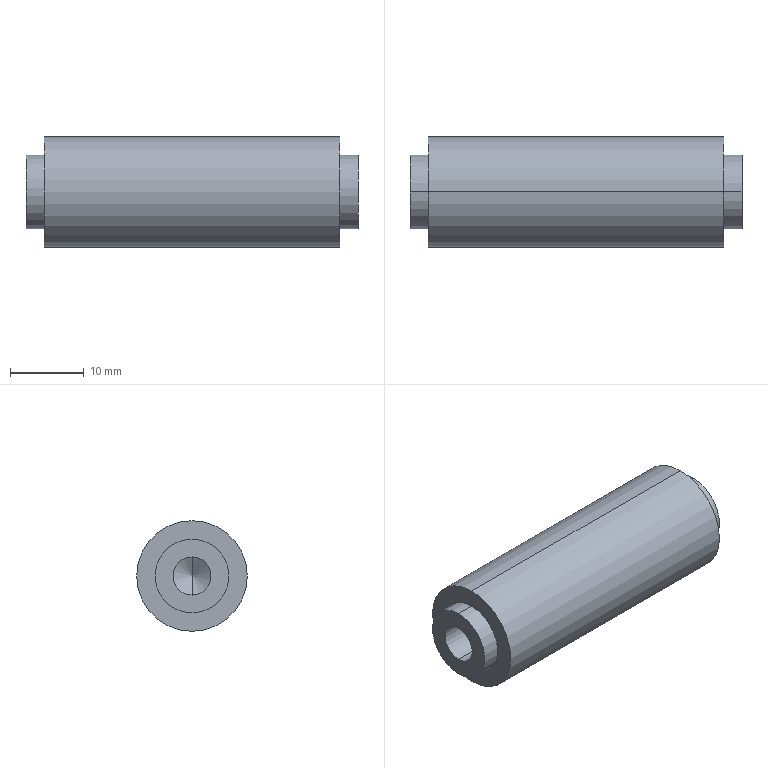Part | SolidWorks | features BaseBody 1 | 1 solid | 18 faces | box 45 x 15 x 15 mm | volume 6805 mm3 | cylinder 10 | cone 4 | plane 4 | commonest cylinder face diameters 5.188 x4 10 x4 15 x2
STEP:
#1=CARTESIAN_POINT('',(20.,0.,7.5));
#2=VERTEX_POINT('',#1);
#3=CARTESIAN_POINT('',(20.,0.,-7.5));
#4=VERTEX_POINT('',#3);
#5=CARTESIAN_POINT('',(20.,0.,0.));
#6=DIRECTION('',(-1.,0.,0.));
#7=DIRECTION('',(0.,0.,1.));
#8=AXIS2_PLACEMENT_3D('',#5,#6,#7);
#9=CIRCLE('',#8,7.5);
#10=EDGE_CURVE('',#2,#4,#9,.T.);
#11=ORIENTED_EDGE('',*,*,#10,.T.);
#12=CARTESIAN_POINT('',(-20.,0.,-7.5));
#13=VERTEX_POINT('',#12);
#14=CARTESIAN_POINT('',(20.,0.,-7.5));
#15=DIRECTION('',(-1.,0.,0.));
#16=VECTOR('',#15,1000.);
#17=LINE('',#14,#16);
#18=EDGE_CURVE('',#4,#13,#17,.T.);
#19=ORIENTED_EDGE('',*,*,#18,.T.);
#20=CARTESIAN_POINT('',(-20.,0.,7.5));
#21=VERTEX_POINT('',#20);
#22=CARTESIAN_POINT('',(-20.,0.,0.));
#23=DIRECTION('',(1.,0.,0.));
#24=DIRECTION('',(0.,0.,1.));
#25=AXIS2_PLACEMENT_3D('',#22,#23,#24);
#26=CIRCLE('',#25,7.5);
#27=EDGE_CURVE('',#13,#21,#26,.T.);
#28=ORIENTED_EDGE('',*,*,#27,.T.);
#29=CARTESIAN_POINT('',(20.,0.,7.5));
#30=DIRECTION('',(-1.,0.,0.));
#31=VECTOR('',#30,1000.);
#32=LINE('',#29,#31);
#33=EDGE_CURVE('',#2,#21,#32,.T.);
#34=ORIENTED_EDGE('',*,*,#33,.F.);
#35=EDGE_LOOP('',(#11,#19,#28,#34));
#36=FACE_OUTER_BOUND('',#35,.T.);
#37=CARTESIAN_POINT('',(20.,0.,0.));
#38=DIRECTION('',(-1.,0.,0.));
#39=DIRECTION('',(0.,0.,1.));
#40=AXIS2_PLACEMENT_3D('',#37,#38,#39);
#41=CYLINDRICAL_SURFACE('',#40,7.5);
#42=ADVANCED_FACE('',(#36),#41,.T.);
#43=CARTESIAN_POINT('',(-20.,0.,5.));
#44=VERTEX_POINT('',#43);
#45=CARTESIAN_POINT('',(-20.,0.,-5.));
#46=VERTEX_POINT('',#45);
#47=CARTESIAN_POINT('',(-20.,0.,0.));
#48=DIRECTION('',(-1.,0.,0.));
#49=DIRECTION('',(0.,0.,1.));
#50=AXIS2_PLACEMENT_3D('',#47,#48,#49);
#51=CIRCLE('',#50,5.);
#52=EDGE_CURVE('',#44,#46,#51,.T.);
#53=ORIENTED_EDGE('',*,*,#52,.T.);
#54=CARTESIAN_POINT('',(-22.5,0.,-5.));
#55=VERTEX_POINT('',#54);
#56=CARTESIAN_POINT('',(-20.,0.,-5.));
#57=DIRECTION('',(-1.,0.,0.));
#58=VECTOR('',#57,1000.);
#59=LINE('',#56,#58);
#60=EDGE_CURVE('',#46,#55,#59,.T.);
#61=ORIENTED_EDGE('',*,*,#60,.T.);
#62=CARTESIAN_POINT('',(-22.5,0.,5.));
#63=VERTEX_POINT('',#62);
#64=CARTESIAN_POINT('',(-22.5,0.,0.));
#65=DIRECTION('',(1.,0.,0.));
#66=DIRECTION('',(0.,0.,1.));
#67=AXIS2_PLACEMENT_3D('',#64,#65,#66);
#68=CIRCLE('',#67,5.);
#69=EDGE_CURVE('',#55,#63,#68,.T.);
#70=ORIENTED_EDGE('',*,*,#69,.T.);
#71=CARTESIAN_POINT('',(-20.,0.,5.));
#72=DIRECTION('',(-1.,0.,0.));
#73=VECTOR('',#72,1000.);
#74=LINE('',#71,#73);
#75=EDGE_CURVE('',#44,#63,#74,.T.);
#76=ORIENTED_EDGE('',*,*,#75,.F.);
#77=EDGE_LOOP('',(#53,#61,#70,#76));
#78=FACE_OUTER_BOUND('',#77,.T.);
#79=CARTESIAN_POINT('',(-20.,0.,0.));
#80=DIRECTION('',(-1.,0.,0.));
#81=DIRECTION('',(0.,0.,1.));
#82=AXIS2_PLACEMENT_3D('',#79,#80,#81);
#83=CYLINDRICAL_SURFACE('',#82,5.);
#84=ADVANCED_FACE('',(#78),#83,.T.);
#85=CARTESIAN_POINT('',(20.,0.,5.));
#86=VERTEX_POINT('',#85);
#87=CARTESIAN_POINT('',(20.,0.,-5.));
#88=VERTEX_POINT('',#87);
#89=CARTESIAN_POINT('',(20.,0.,0.));
#90=DIRECTION('',(-1.,0.,0.));
#91=DIRECTION('',(0.,0.,-1.));
#92=AXIS2_PLACEMENT_3D('',#89,#90,#91);
#93=CIRCLE('',#92,5.);
#94=EDGE_CURVE('',#86,#88,#93,.T.);
#95=ORIENTED_EDGE('',*,*,#94,.F.);
#96=CARTESIAN_POINT('',(22.5,0.,5.));
#97=VERTEX_POINT('',#96);
#98=CARTESIAN_POINT('',(20.,0.,5.));
#99=DIRECTION('',(1.,0.,0.));
#100=VECTOR('',#99,1000.);
#101=LINE('',#98,#100);
#102=EDGE_CURVE('',#86,#97,#101,.T.);
#103=ORIENTED_EDGE('',*,*,#102,.T.);
#104=CARTESIAN_POINT('',(22.5,0.,-5.));
#105=VERTEX_POINT('',#104);
#106=CARTESIAN_POINT('',(22.5,0.,0.));
#107=DIRECTION('',(-1.,0.,0.));
#108=DIRECTION('',(0.,0.,-1.));
#109=AXIS2_PLACEMENT_3D('',#106,#107,#108);
#110=CIRCLE('',#109,5.);
#111=EDGE_CURVE('',#97,#105,#110,.T.);
#112=ORIENTED_EDGE('',*,*,#111,.T.);
#113=CARTESIAN_POINT('',(20.,0.,-5.));
#114=DIRECTION('',(1.,0.,0.));
#115=VECTOR('',#114,1000.);
#116=LINE('',#113,#115);
#117=EDGE_CURVE('',#88,#105,#116,.T.);
#118=ORIENTED_EDGE('',*,*,#117,.F.);
#119=EDGE_LOOP('',(#95,#103,#112,#118));
#120=FACE_OUTER_BOUND('',#119,.T.);
#121=CARTESIAN_POINT('',(20.,0.,0.));
#122=DIRECTION('',(1.,0.,0.));
#123=DIRECTION('',(0.,0.,-1.));
#124=AXIS2_PLACEMENT_3D('',#121,#122,#123);
#125=CYLINDRICAL_SURFACE('',#124,5.);
#126=ADVANCED_FACE('',(#120),#125,.T.);
#127=CARTESIAN_POINT('',(-22.5,0.,2.594));
#128=VERTEX_POINT('',#127);
#129=CARTESIAN_POINT('',(-22.5,0.,-2.594));
#130=VERTEX_POINT('',#129);
#131=CARTESIAN_POINT('',(-22.5,0.,0.));
#132=DIRECTION('',(1.,0.,0.));
#133=DIRECTION('',(0.,0.,-1.));
#134=AXIS2_PLACEMENT_3D('',#131,#132,#133);
#135=CIRCLE('',#134,2.594);
#136=EDGE_CURVE('',#128,#130,#135,.T.);
#137=ORIENTED_EDGE('',*,*,#136,.F.);
#138=CARTESIAN_POINT('',(-7.5,0.,2.594));
#139=VERTEX_POINT('',#138);
#140=CARTESIAN_POINT('',(-22.5,0.,2.594));
#141=DIRECTION('',(1.,0.,0.));
#142=VECTOR('',#141,1000.);
#143=LINE('',#140,#142);
#144=EDGE_CURVE('',#128,#139,#143,.T.);
#145=ORIENTED_EDGE('',*,*,#144,.T.);
#146=CARTESIAN_POINT('',(-7.5,0.,-2.594));
#147=VERTEX_POINT('',#146);
#148=CARTESIAN_POINT('',(-7.5,0.,0.));
#149=DIRECTION('',(-1.,0.,0.));
#150=DIRECTION('',(0.,0.,-1.));
#151=AXIS2_PLACEMENT_3D('',#148,#149,#150);
#152=CIRCLE('',#151,2.594);
#153=EDGE_CURVE('',#147,#139,#152,.T.);
#154=ORIENTED_EDGE('',*,*,#153,.F.);
#155=CARTESIAN_POINT('',(-22.5,0.,-2.594));
#156=DIRECTION('',(1.,0.,0.));
#157=VECTOR('',#156,1000.);
#158=LINE('',#155,#157);
#159=EDGE_CURVE('',#130,#147,#158,.T.);
#160=ORIENTED_EDGE('',*,*,#159,.F.);
#161=EDGE_LOOP('',(#137,#145,#154,#160));
#162=FACE_OUTER_BOUND('',#161,.T.);
#163=CARTESIAN_POINT('',(-22.5,0.,0.));
#164=DIRECTION('',(1.,0.,0.));
#165=DIRECTION('',(0.,0.,-1.));
#166=AXIS2_PLACEMENT_3D('',#163,#164,#165);
#167=CYLINDRICAL_SURFACE('',#166,2.594);
#168=ADVANCED_FACE('',(#162),#167,.F.);
#169=CARTESIAN_POINT('',(22.5,0.,-2.594));
#170=VERTEX_POINT('',#169);
#171=CARTESIAN_POINT('',(22.5,0.,2.594));
#172=VERTEX_POINT('',#171);
#173=CARTESIAN_POINT('',(22.5,0.,0.));
#174=DIRECTION('',(-1.,0.,0.));
#175=DIRECTION('',(0.,0.,1.));
#176=AXIS2_PLACEMENT_3D('',#173,#174,#175);
#177=CIRCLE('',#176,2.594);
#178=EDGE_CURVE('',#170,#172,#177,.T.);
#179=ORIENTED_EDGE('',*,*,#178,.F.);
#180=CARTESIAN_POINT('',(7.5,0.,-2.594));
#181=VERTEX_POINT('',#180);
#182=CARTESIAN_POINT('',(22.5,0.,-2.594));
#183=DIRECTION('',(-1.,0.,0.));
#184=VECTOR('',#183,1000.);
#185=LINE('',#182,#184);
#186=EDGE_CURVE('',#170,#181,#185,.T.);
#187=ORIENTED_EDGE('',*,*,#186,.T.);
#188=CARTESIAN_POINT('',(7.5,0.,2.594));
#189=VERTEX_POINT('',#188);
#190=CARTESIAN_POINT('',(7.5,0.,0.));
#191=DIRECTION('',(1.,0.,0.));
#192=DIRECTION('',(0.,0.,1.));
#193=AXIS2_PLACEMENT_3D('',#190,#191,#192);
#194=CIRCLE('',#193,2.594);
#195=EDGE_CURVE('',#189,#181,#194,.T.);
#196=ORIENTED_EDGE('',*,*,#195,.F.);
#197=CARTESIAN_POINT('',(22.5,0.,2.594));
#198=DIRECTION('',(-1.,0.,0.));
#199=VECTOR('',#198,1000.);
#200=LINE('',#197,#199);
#201=EDGE_CURVE('',#172,#189,#200,.T.);
#202=ORIENTED_EDGE('',*,*,#201,.F.);
#203=EDGE_LOOP('',(#179,#187,#196,#202));
#204=FACE_OUTER_BOUND('',#203,.T.);
#205=CARTESIAN_POINT('',(22.5,0.,0.));
#206=DIRECTION('',(-1.,0.,0.));
#207=DIRECTION('',(0.,0.,1.));
#208=AXIS2_PLACEMENT_3D('',#205,#206,#207);
#209=CYLINDRICAL_SURFACE('',#208,2.594);
#210=ADVANCED_FACE('',(#204),#209,.F.);
#211=CARTESIAN_POINT('',(-5.941,0.,0.));
#212=VERTEX_POINT('',#211);
#213=CARTESIAN_POINT('',(-7.5,0.,2.594));
#214=DIRECTION('',(-0.515,0.,0.8572));
#215=VECTOR('',#214,1000.);
#216=LINE('',#213,#215);
#217=EDGE_CURVE('',#212,#139,#216,.T.);
#218=ORIENTED_EDGE('',*,*,#217,.F.);
#219=CARTESIAN_POINT('',(-7.5,0.,-2.594));
#220=DIRECTION('',(-0.515,0.,-0.8572));
#221=VECTOR('',#220,1000.);
#222=LINE('',#219,#221);
#223=EDGE_CURVE('',#212,#147,#222,.T.);
#224=ORIENTED_EDGE('',*,*,#223,.T.);
#225=ORIENTED_EDGE('',*,*,#153,.T.);
#226=EDGE_LOOP('',(#218,#224,#225));
#227=FACE_OUTER_BOUND('',#226,.T.);
#228=CARTESIAN_POINT('',(-7.5,0.,0.));
#229=DIRECTION('',(-1.,0.,0.));
#230=DIRECTION('',(0.,0.,1.));
#231=AXIS2_PLACEMENT_3D('',#228,#229,#230);
#232=CONICAL_SURFACE('',#231,2.594,1.03);
#233=ADVANCED_FACE('',(#227),#232,.F.);
#234=CARTESIAN_POINT('',(5.941,0.,0.));
#235=VERTEX_POINT('',#234);
#236=CARTESIAN_POINT('',(7.5,0.,-2.594));
#237=DIRECTION('',(0.515,0.,-0.8572));
#238=VECTOR('',#237,1000.);
#239=LINE('',#236,#238);
#240=EDGE_CURVE('',#235,#181,#239,.T.);
#241=ORIENTED_EDGE('',*,*,#240,.F.);
#242=CARTESIAN_POINT('',(7.5,0.,2.594));
#243=DIRECTION('',(0.515,0.,0.8572));
#244=VECTOR('',#243,1000.);
#245=LINE('',#242,#244);
#246=EDGE_CURVE('',#235,#189,#245,.T.);
#247=ORIENTED_EDGE('',*,*,#246,.T.);
#248=ORIENTED_EDGE('',*,*,#195,.T.);
#249=EDGE_LOOP('',(#241,#247,#248));
#250=FACE_OUTER_BOUND('',#249,.T.);
#251=CARTESIAN_POINT('',(7.5,0.,0.));
#252=DIRECTION('',(1.,0.,0.));
#253=DIRECTION('',(0.,0.,-1.));
#254=AXIS2_PLACEMENT_3D('',#251,#252,#253);
#255=CONICAL_SURFACE('',#254,2.594,1.03);
#256=ADVANCED_FACE('',(#250),#255,.F.);
#257=ORIENTED_EDGE('',*,*,#18,.F.);
#258=CARTESIAN_POINT('',(20.,0.,0.));
#259=DIRECTION('',(-1.,0.,0.));
#260=DIRECTION('',(0.,0.,1.));
#261=AXIS2_PLACEMENT_3D('',#258,#259,#260);
#262=CIRCLE('',#261,7.5);
#263=EDGE_CURVE('',#4,#2,#262,.T.);
#264=ORIENTED_EDGE('',*,*,#263,.T.);
#265=ORIENTED_EDGE('',*,*,#33,.T.);
#266=CARTESIAN_POINT('',(-20.,0.,0.));
#267=DIRECTION('',(1.,0.,0.));
#268=DIRECTION('',(0.,0.,1.));
#269=AXIS2_PLACEMENT_3D('',#266,#267,#268);
#270=CIRCLE('',#269,7.5);
#271=EDGE_CURVE('',#21,#13,#270,.T.);
#272=ORIENTED_EDGE('',*,*,#271,.T.);
#273=EDGE_LOOP('',(#257,#264,#265,#272));
#274=FACE_OUTER_BOUND('',#273,.T.);
#275=CARTESIAN_POINT('',(20.,0.,0.));
#276=DIRECTION('',(-1.,0.,0.));
#277=DIRECTION('',(0.,0.,1.));
#278=AXIS2_PLACEMENT_3D('',#275,#276,#277);
#279=CYLINDRICAL_SURFACE('',#278,7.5);
#280=ADVANCED_FACE('',(#274),#279,.T.);
#281=ORIENTED_EDGE('',*,*,#271,.F.);
#282=ORIENTED_EDGE('',*,*,#27,.F.);
#283=EDGE_LOOP('',(#281,#282));
#284=FACE_OUTER_BOUND('',#283,.T.);
#285=ORIENTED_EDGE('',*,*,#52,.F.);
#286=CARTESIAN_POINT('',(-20.,0.,0.));
#287=DIRECTION('',(-1.,0.,0.));
#288=DIRECTION('',(0.,0.,1.));
#289=AXIS2_PLACEMENT_3D('',#286,#287,#288);
#290=CIRCLE('',#289,5.);
#291=EDGE_CURVE('',#46,#44,#290,.T.);
#292=ORIENTED_EDGE('',*,*,#291,.F.);
#293=EDGE_LOOP('',(#285,#292));
#294=FACE_BOUND('',#293,.T.);
#295=CARTESIAN_POINT('',(-20.,0.,0.));
#296=DIRECTION('',(1.,0.,0.));
#297=DIRECTION('',(0.,0.,-1.));
#298=AXIS2_PLACEMENT_3D('',#295,#296,#297);
#299=PLANE('',#298);
#300=ADVANCED_FACE('',(#284,#294),#299,.F.);
#301=ORIENTED_EDGE('',*,*,#10,.F.);
#302=ORIENTED_EDGE('',*,*,#263,.F.);
#303=EDGE_LOOP('',(#301,#302));
#304=FACE_OUTER_BOUND('',#303,.T.);
#305=CARTESIAN_POINT('',(20.,0.,0.));
#306=DIRECTION('',(-1.,0.,0.));
#307=DIRECTION('',(0.,0.,-1.));
#308=AXIS2_PLACEMENT_3D('',#305,#306,#307);
#309=CIRCLE('',#308,5.);
#310=EDGE_CURVE('',#88,#86,#309,.T.);
#311=ORIENTED_EDGE('',*,*,#310,.T.);
#312=ORIENTED_EDGE('',*,*,#94,.T.);
#313=EDGE_LOOP('',(#311,#312));
#314=FACE_BOUND('',#313,.T.);
#315=CARTESIAN_POINT('',(20.,0.,0.));
#316=DIRECTION('',(1.,0.,0.));
#317=DIRECTION('',(0.,0.,-1.));
#318=AXIS2_PLACEMENT_3D('',#315,#316,#317);
#319=PLANE('',#318);
#320=ADVANCED_FACE('',(#304,#314),#319,.T.);
#321=ORIENTED_EDGE('',*,*,#60,.F.);
#322=ORIENTED_EDGE('',*,*,#291,.T.);
#323=ORIENTED_EDGE('',*,*,#75,.T.);
#324=CARTESIAN_POINT('',(-22.5,0.,0.));
#325=DIRECTION('',(1.,0.,0.));
#326=DIRECTION('',(0.,0.,1.));
#327=AXIS2_PLACEMENT_3D('',#324,#325,#326);
#328=CIRCLE('',#327,5.);
#329=EDGE_CURVE('',#63,#55,#328,.T.);
#330=ORIENTED_EDGE('',*,*,#329,.T.);
#331=EDGE_LOOP('',(#321,#322,#323,#330));
#332=FACE_OUTER_BOUND('',#331,.T.);
#333=CARTESIAN_POINT('',(-20.,0.,0.));
#334=DIRECTION('',(-1.,0.,0.));
#335=DIRECTION('',(0.,0.,1.));
#336=AXIS2_PLACEMENT_3D('',#333,#334,#335);
#337=CYLINDRICAL_SURFACE('',#336,5.);
#338=ADVANCED_FACE('',(#332),#337,.T.);
#339=ORIENTED_EDGE('',*,*,#102,.F.);
#340=ORIENTED_EDGE('',*,*,#310,.F.);
#341=ORIENTED_EDGE('',*,*,#117,.T.);
#342=CARTESIAN_POINT('',(22.5,0.,0.));
#343=DIRECTION('',(-1.,0.,0.));
#344=DIRECTION('',(0.,0.,-1.));
#345=AXIS2_PLACEMENT_3D('',#342,#343,#344);
#346=CIRCLE('',#345,5.);
#347=EDGE_CURVE('',#105,#97,#346,.T.);
#348=ORIENTED_EDGE('',*,*,#347,.T.);
#349=EDGE_LOOP('',(#339,#340,#341,#348));
#350=FACE_OUTER_BOUND('',#349,.T.);
#351=CARTESIAN_POINT('',(20.,0.,0.));
#352=DIRECTION('',(1.,0.,0.));
#353=DIRECTION('',(0.,0.,-1.));
#354=AXIS2_PLACEMENT_3D('',#351,#352,#353);
#355=CYLINDRICAL_SURFACE('',#354,5.);
#356=ADVANCED_FACE('',(#350),#355,.T.);
#357=ORIENTED_EDGE('',*,*,#329,.F.);
#358=ORIENTED_EDGE('',*,*,#69,.F.);
#359=EDGE_LOOP('',(#357,#358));
#360=FACE_OUTER_BOUND('',#359,.T.);
#361=CARTESIAN_POINT('',(-22.5,0.,0.));
#362=DIRECTION('',(1.,0.,0.));
#363=DIRECTION('',(0.,0.,-1.));
#364=AXIS2_PLACEMENT_3D('',#361,#362,#363);
#365=CIRCLE('',#364,2.594);
#366=EDGE_CURVE('',#130,#128,#365,.T.);
#367=ORIENTED_EDGE('',*,*,#366,.T.);
#368=ORIENTED_EDGE('',*,*,#136,.T.);
#369=EDGE_LOOP('',(#367,#368));
#370=FACE_BOUND('',#369,.T.);
#371=CARTESIAN_POINT('',(-22.5,0.,0.));
#372=DIRECTION('',(-1.,0.,0.));
#373=DIRECTION('',(0.,0.,1.));
#374=AXIS2_PLACEMENT_3D('',#371,#372,#373);
#375=PLANE('',#374);
#376=ADVANCED_FACE('',(#360,#370),#375,.T.);
#377=ORIENTED_EDGE('',*,*,#347,.F.);
#378=ORIENTED_EDGE('',*,*,#111,.F.);
#379=EDGE_LOOP('',(#377,#378));
#380=FACE_OUTER_BOUND('',#379,.T.);
#381=CARTESIAN_POINT('',(22.5,0.,0.));
#382=DIRECTION('',(-1.,0.,0.));
#383=DIRECTION('',(0.,0.,1.));
#384=AXIS2_PLACEMENT_3D('',#381,#382,#383);
#385=CIRCLE('',#384,2.594);
#386=EDGE_CURVE('',#172,#170,#385,.T.);
#387=ORIENTED_EDGE('',*,*,#386,.T.);
#388=ORIENTED_EDGE('',*,*,#178,.T.);
#389=EDGE_LOOP('',(#387,#388));
#390=FACE_BOUND('',#389,.T.);
#391=CARTESIAN_POINT('',(22.5,0.,0.));
#392=DIRECTION('',(1.,0.,0.));
#393=DIRECTION('',(0.,0.,-1.));
#394=AXIS2_PLACEMENT_3D('',#391,#392,#393);
#395=PLANE('',#394);
#396=ADVANCED_FACE('',(#380,#390),#395,.T.);
#397=ORIENTED_EDGE('',*,*,#144,.F.);
#398=ORIENTED_EDGE('',*,*,#366,.F.);
#399=ORIENTED_EDGE('',*,*,#159,.T.);
#400=CARTESIAN_POINT('',(-7.5,0.,0.));
#401=DIRECTION('',(-1.,0.,0.));
#402=DIRECTION('',(0.,0.,-1.));
#403=AXIS2_PLACEMENT_3D('',#400,#401,#402);
#404=CIRCLE('',#403,2.594);
#405=EDGE_CURVE('',#139,#147,#404,.T.);
#406=ORIENTED_EDGE('',*,*,#405,.F.);
#407=EDGE_LOOP('',(#397,#398,#399,#406));
#408=FACE_OUTER_BOUND('',#407,.T.);
#409=CARTESIAN_POINT('',(-22.5,0.,0.));
#410=DIRECTION('',(1.,0.,0.));
#411=DIRECTION('',(0.,0.,-1.));
#412=AXIS2_PLACEMENT_3D('',#409,#410,#411);
#413=CYLINDRICAL_SURFACE('',#412,2.594);
#414=ADVANCED_FACE('',(#408),#413,.F.);
#415=ORIENTED_EDGE('',*,*,#186,.F.);
#416=ORIENTED_EDGE('',*,*,#386,.F.);
#417=ORIENTED_EDGE('',*,*,#201,.T.);
#418=CARTESIAN_POINT('',(7.5,0.,0.));
#419=DIRECTION('',(1.,0.,0.));
#420=DIRECTION('',(0.,0.,1.));
#421=AXIS2_PLACEMENT_3D('',#418,#419,#420);
#422=CIRCLE('',#421,2.594);
#423=EDGE_CURVE('',#181,#189,#422,.T.);
#424=ORIENTED_EDGE('',*,*,#423,.F.);
#425=EDGE_LOOP('',(#415,#416,#417,#424));
#426=FACE_OUTER_BOUND('',#425,.T.);
#427=CARTESIAN_POINT('',(22.5,0.,0.));
#428=DIRECTION('',(-1.,0.,0.));
#429=DIRECTION('',(0.,0.,1.));
#430=AXIS2_PLACEMENT_3D('',#427,#428,#429);
#431=CYLINDRICAL_SURFACE('',#430,2.594);
#432=ADVANCED_FACE('',(#426),#431,.F.);
#433=ORIENTED_EDGE('',*,*,#223,.F.);
#434=ORIENTED_EDGE('',*,*,#217,.T.);
#435=ORIENTED_EDGE('',*,*,#405,.T.);
#436=EDGE_LOOP('',(#433,#434,#435));
#437=FACE_OUTER_BOUND('',#436,.T.);
#438=CARTESIAN_POINT('',(-7.5,0.,0.));
#439=DIRECTION('',(-1.,0.,0.));
#440=DIRECTION('',(0.,0.,1.));
#441=AXIS2_PLACEMENT_3D('',#438,#439,#440);
#442=CONICAL_SURFACE('',#441,2.594,1.03);
#443=ADVANCED_FACE('',(#437),#442,.F.);
#444=ORIENTED_EDGE('',*,*,#246,.F.);
#445=ORIENTED_EDGE('',*,*,#240,.T.);
#446=ORIENTED_EDGE('',*,*,#423,.T.);
#447=EDGE_LOOP('',(#444,#445,#446));
#448=FACE_OUTER_BOUND('',#447,.T.);
#449=CARTESIAN_POINT('',(7.5,0.,0.));
#450=DIRECTION('',(1.,0.,0.));
#451=DIRECTION('',(0.,0.,-1.));
#452=AXIS2_PLACEMENT_3D('',#449,#450,#451);
#453=CONICAL_SURFACE('',#452,2.594,1.03);
#454=ADVANCED_FACE('',(#448),#453,.F.);
#455=CLOSED_SHELL('',(#42,#84,#126,#168,#210,#233,#256,#280,#300,#320,#338,#356,#376,#396,#414,#432,#443,#454));
#456=MANIFOLD_SOLID_BREP('',#455);
#457=CARTESIAN_POINT('',(0.,0.,0.));
#458=DIRECTION('',(0.,0.,1.));
#459=DIRECTION('',(1.,0.,0.));
#460=AXIS2_PLACEMENT_3D('',#457,#458,#459);
#461=(LENGTH_UNIT()NAMED_UNIT(*)SI_UNIT(.MILLI.,.METRE.));
#462=UNCERTAINTY_MEASURE_WITH_UNIT(LENGTH_MEASURE(0.00001),#461,'','');
#463=(NAMED_UNIT(*)PLANE_ANGLE_UNIT()SI_UNIT($,.RADIAN.));
#464=(NAMED_UNIT(*)SI_UNIT($,.STERADIAN.)SOLID_ANGLE_UNIT());
#465=(GEOMETRIC_REPRESENTATION_CONTEXT(3)GLOBAL_UNCERTAINTY_ASSIGNED_CONTEXT((#462))GLOBAL_UNIT_ASSIGNED_CONTEXT((#461,#463,#464))REPRESENTATION_CONTEXT('',''));
#466=ADVANCED_BREP_SHAPE_REPRESENTATION('',(#456,#460),#465);